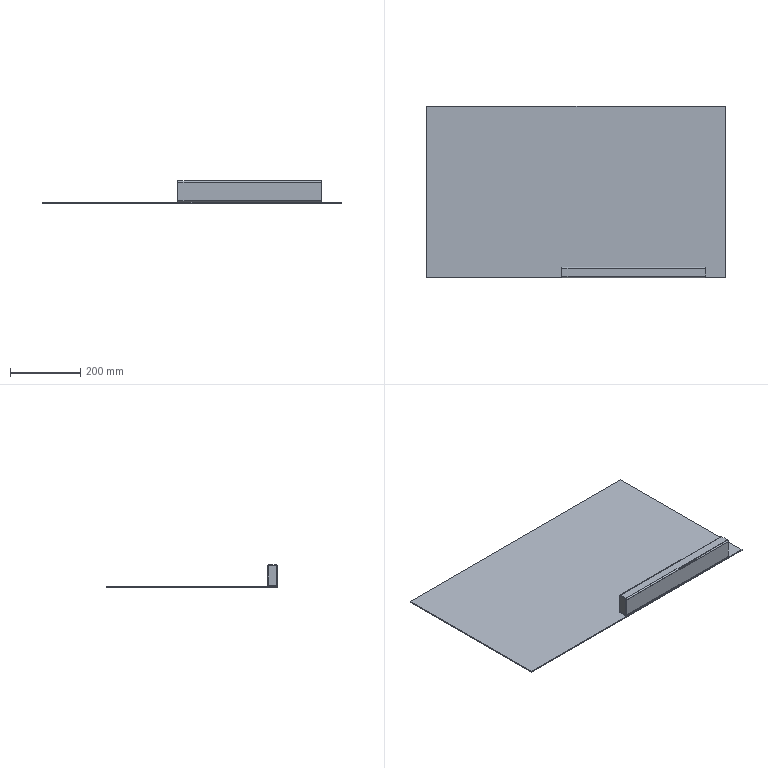Part | SolidWorks | features EndCap 1, Extrusion 1, WeldMemberFeat 1, WeldmentFeature 1 | 3 solids | 34 faces | box 850 x 488 x 63 mm | volume 1385283 mm3 | plane 22 | cylinder 12 | commonest cylinder face diameters 4 x8 8 x4
STEP:
#1=CARTESIAN_POINT('',(425.,-244.,-1.5));
#2=VERTEX_POINT('',#1);
#3=CARTESIAN_POINT('',(425.,244.,-1.5));
#4=VERTEX_POINT('',#3);
#5=CARTESIAN_POINT('',(425.,244.,-1.5));
#6=DIRECTION('',(0.,1.,0.));
#7=VECTOR('',#6,1000.);
#8=LINE('',#5,#7);
#9=EDGE_CURVE('',#2,#4,#8,.T.);
#10=ORIENTED_EDGE('',*,*,#9,.T.);
#11=CARTESIAN_POINT('',(425.,244.,1.5));
#12=VERTEX_POINT('',#11);
#13=CARTESIAN_POINT('',(425.,244.,1.5));
#14=DIRECTION('',(0.,0.,-1.));
#15=VECTOR('',#14,1000.);
#16=LINE('',#13,#15);
#17=EDGE_CURVE('',#12,#4,#16,.T.);
#18=ORIENTED_EDGE('',*,*,#17,.F.);
#19=CARTESIAN_POINT('',(425.,-244.,1.5));
#20=VERTEX_POINT('',#19);
#21=CARTESIAN_POINT('',(425.,244.,1.5));
#22=DIRECTION('',(0.,1.,0.));
#23=VECTOR('',#22,1000.);
#24=LINE('',#21,#23);
#25=EDGE_CURVE('',#20,#12,#24,.T.);
#26=ORIENTED_EDGE('',*,*,#25,.F.);
#27=CARTESIAN_POINT('',(425.,-244.,1.5));
#28=DIRECTION('',(0.,0.,-1.));
#29=VECTOR('',#28,1000.);
#30=LINE('',#27,#29);
#31=EDGE_CURVE('',#20,#2,#30,.T.);
#32=ORIENTED_EDGE('',*,*,#31,.T.);
#33=EDGE_LOOP('',(#10,#18,#26,#32));
#34=FACE_OUTER_BOUND('',#33,.T.);
#35=CARTESIAN_POINT('',(425.,244.,1.5));
#36=DIRECTION('',(-1.,0.,0.));
#37=DIRECTION('',(0.,-1.,0.));
#38=AXIS2_PLACEMENT_3D('',#35,#36,#37);
#39=PLANE('',#38);
#40=ADVANCED_FACE('',(#34),#39,.F.);
#41=CARTESIAN_POINT('',(-425.,244.,-1.5));
#42=VERTEX_POINT('',#41);
#43=CARTESIAN_POINT('',(-425.,244.,-1.5));
#44=DIRECTION('',(-1.,0.,0.));
#45=VECTOR('',#44,1000.);
#46=LINE('',#43,#45);
#47=EDGE_CURVE('',#4,#42,#46,.T.);
#48=ORIENTED_EDGE('',*,*,#47,.T.);
#49=CARTESIAN_POINT('',(-425.,244.,1.5));
#50=VERTEX_POINT('',#49);
#51=CARTESIAN_POINT('',(-425.,244.,1.5));
#52=DIRECTION('',(0.,0.,-1.));
#53=VECTOR('',#52,1000.);
#54=LINE('',#51,#53);
#55=EDGE_CURVE('',#50,#42,#54,.T.);
#56=ORIENTED_EDGE('',*,*,#55,.F.);
#57=CARTESIAN_POINT('',(-425.,244.,1.5));
#58=DIRECTION('',(-1.,0.,0.));
#59=VECTOR('',#58,1000.);
#60=LINE('',#57,#59);
#61=EDGE_CURVE('',#12,#50,#60,.T.);
#62=ORIENTED_EDGE('',*,*,#61,.F.);
#63=ORIENTED_EDGE('',*,*,#17,.T.);
#64=EDGE_LOOP('',(#48,#56,#62,#63));
#65=FACE_OUTER_BOUND('',#64,.T.);
#66=CARTESIAN_POINT('',(-425.,244.,1.5));
#67=DIRECTION('',(0.,-1.,0.));
#68=DIRECTION('',(0.,0.,-1.));
#69=AXIS2_PLACEMENT_3D('',#66,#67,#68);
#70=PLANE('',#69);
#71=ADVANCED_FACE('',(#65),#70,.F.);
#72=CARTESIAN_POINT('',(-425.,-244.,-1.5));
#73=VERTEX_POINT('',#72);
#74=CARTESIAN_POINT('',(-425.,244.,-1.5));
#75=DIRECTION('',(0.,-1.,0.));
#76=VECTOR('',#75,1000.);
#77=LINE('',#74,#76);
#78=EDGE_CURVE('',#42,#73,#77,.T.);
#79=ORIENTED_EDGE('',*,*,#78,.T.);
#80=CARTESIAN_POINT('',(-425.,-244.,1.5));
#81=VERTEX_POINT('',#80);
#82=CARTESIAN_POINT('',(-425.,-244.,1.5));
#83=DIRECTION('',(0.,0.,-1.));
#84=VECTOR('',#83,1000.);
#85=LINE('',#82,#84);
#86=EDGE_CURVE('',#81,#73,#85,.T.);
#87=ORIENTED_EDGE('',*,*,#86,.F.);
#88=CARTESIAN_POINT('',(-425.,244.,1.5));
#89=DIRECTION('',(0.,-1.,0.));
#90=VECTOR('',#89,1000.);
#91=LINE('',#88,#90);
#92=EDGE_CURVE('',#50,#81,#91,.T.);
#93=ORIENTED_EDGE('',*,*,#92,.F.);
#94=ORIENTED_EDGE('',*,*,#55,.T.);
#95=EDGE_LOOP('',(#79,#87,#93,#94));
#96=FACE_OUTER_BOUND('',#95,.T.);
#97=CARTESIAN_POINT('',(-425.,244.,1.5));
#98=DIRECTION('',(1.,0.,0.));
#99=DIRECTION('',(0.,1.,0.));
#100=AXIS2_PLACEMENT_3D('',#97,#98,#99);
#101=PLANE('',#100);
#102=ADVANCED_FACE('',(#96),#101,.F.);
#103=CARTESIAN_POINT('',(-425.,-244.,-1.5));
#104=DIRECTION('',(1.,0.,0.));
#105=VECTOR('',#104,1000.);
#106=LINE('',#103,#105);
#107=EDGE_CURVE('',#73,#2,#106,.T.);
#108=ORIENTED_EDGE('',*,*,#107,.T.);
#109=ORIENTED_EDGE('',*,*,#31,.F.);
#110=CARTESIAN_POINT('',(-425.,-244.,1.5));
#111=DIRECTION('',(1.,0.,0.));
#112=VECTOR('',#111,1000.);
#113=LINE('',#110,#112);
#114=EDGE_CURVE('',#81,#20,#113,.T.);
#115=ORIENTED_EDGE('',*,*,#114,.F.);
#116=ORIENTED_EDGE('',*,*,#86,.T.);
#117=EDGE_LOOP('',(#108,#109,#115,#116));
#118=FACE_OUTER_BOUND('',#117,.T.);
#119=CARTESIAN_POINT('',(-425.,-244.,1.5));
#120=DIRECTION('',(0.,1.,0.));
#121=DIRECTION('',(0.,0.,1.));
#122=AXIS2_PLACEMENT_3D('',#119,#120,#121);
#123=PLANE('',#122);
#124=ADVANCED_FACE('',(#118),#123,.F.);
#125=ORIENTED_EDGE('',*,*,#25,.T.);
#126=ORIENTED_EDGE('',*,*,#61,.T.);
#127=ORIENTED_EDGE('',*,*,#92,.T.);
#128=ORIENTED_EDGE('',*,*,#114,.T.);
#129=EDGE_LOOP('',(#125,#126,#127,#128));
#130=FACE_OUTER_BOUND('',#129,.T.);
#131=CARTESIAN_POINT('',(0.,0.,1.5));
#132=DIRECTION('',(0.,0.,1.));
#133=DIRECTION('',(1.,0.,0.));
#134=AXIS2_PLACEMENT_3D('',#131,#132,#133);
#135=PLANE('',#134);
#136=ADVANCED_FACE('',(#130),#135,.T.);
#137=ORIENTED_EDGE('',*,*,#9,.F.);
#138=ORIENTED_EDGE('',*,*,#107,.F.);
#139=ORIENTED_EDGE('',*,*,#78,.F.);
#140=ORIENTED_EDGE('',*,*,#47,.F.);
#141=EDGE_LOOP('',(#137,#138,#139,#140));
#142=FACE_OUTER_BOUND('',#141,.T.);
#143=CARTESIAN_POINT('',(0.,0.,-1.5));
#144=DIRECTION('',(0.,0.,1.));
#145=DIRECTION('',(1.,0.,0.));
#146=AXIS2_PLACEMENT_3D('',#143,#144,#145);
#147=PLANE('',#146);
#148=ADVANCED_FACE('',(#142),#147,.F.);
#149=CLOSED_SHELL('',(#40,#71,#102,#124,#136,#148));
#150=MANIFOLD_SOLID_BREP('',#149);
#151=CARTESIAN_POINT('',(370.,-244.,57.5));
#152=VERTEX_POINT('',#151);
#153=CARTESIAN_POINT('',(370.,-240.,61.5));
#154=VERTEX_POINT('',#153);
#155=CARTESIAN_POINT('',(370.,-240.,57.5));
#156=DIRECTION('',(-1.,0.,0.));
#157=DIRECTION('',(0.,-1.,0.));
#158=AXIS2_PLACEMENT_3D('',#155,#156,#157);
#159=CIRCLE('',#158,4.);
#160=EDGE_CURVE('',#152,#154,#159,.T.);
#161=ORIENTED_EDGE('',*,*,#160,.T.);
#162=CARTESIAN_POINT('',(-40.,-240.,61.5));
#163=VERTEX_POINT('',#162);
#164=CARTESIAN_POINT('',(-40.,-240.,61.5));
#165=DIRECTION('',(1.,0.,0.));
#166=VECTOR('',#165,1000.);
#167=LINE('',#164,#166);
#168=EDGE_CURVE('',#163,#154,#167,.T.);
#169=ORIENTED_EDGE('',*,*,#168,.F.);
#170=CARTESIAN_POINT('',(-40.,-244.,57.5));
#171=VERTEX_POINT('',#170);
#172=CARTESIAN_POINT('',(-40.,-240.,57.5));
#173=DIRECTION('',(-1.,0.,0.));
#174=DIRECTION('',(0.,-1.,0.));
#175=AXIS2_PLACEMENT_3D('',#172,#173,#174);
#176=CIRCLE('',#175,4.);
#177=EDGE_CURVE('',#171,#163,#176,.T.);
#178=ORIENTED_EDGE('',*,*,#177,.F.);
#179=CARTESIAN_POINT('',(-40.,-244.,57.5));
#180=DIRECTION('',(1.,0.,0.));
#181=VECTOR('',#180,1000.);
#182=LINE('',#179,#181);
#183=EDGE_CURVE('',#171,#152,#182,.T.);
#184=ORIENTED_EDGE('',*,*,#183,.T.);
#185=EDGE_LOOP('',(#161,#169,#178,#184));
#186=FACE_OUTER_BOUND('',#185,.T.);
#187=CARTESIAN_POINT('',(-40.,-240.,57.5));
#188=DIRECTION('',(1.,0.,0.));
#189=DIRECTION('',(0.,1.,0.));
#190=AXIS2_PLACEMENT_3D('',#187,#188,#189);
#191=CYLINDRICAL_SURFACE('',#190,4.);
#192=ADVANCED_FACE('',(#186),#191,.T.);
#193=CARTESIAN_POINT('',(370.,-218.,61.5));
#194=VERTEX_POINT('',#193);
#195=CARTESIAN_POINT('',(370.,-240.,61.5));
#196=DIRECTION('',(0.,1.,0.));
#197=VECTOR('',#196,1000.);
#198=LINE('',#195,#197);
#199=EDGE_CURVE('',#154,#194,#198,.T.);
#200=ORIENTED_EDGE('',*,*,#199,.T.);
#201=CARTESIAN_POINT('',(-40.,-218.,61.5));
#202=VERTEX_POINT('',#201);
#203=CARTESIAN_POINT('',(-40.,-218.,61.5));
#204=DIRECTION('',(1.,0.,0.));
#205=VECTOR('',#204,1000.);
#206=LINE('',#203,#205);
#207=EDGE_CURVE('',#202,#194,#206,.T.);
#208=ORIENTED_EDGE('',*,*,#207,.F.);
#209=CARTESIAN_POINT('',(-40.,-240.,61.5));
#210=DIRECTION('',(0.,1.,0.));
#211=VECTOR('',#210,1000.);
#212=LINE('',#209,#211);
#213=EDGE_CURVE('',#163,#202,#212,.T.);
#214=ORIENTED_EDGE('',*,*,#213,.F.);
#215=ORIENTED_EDGE('',*,*,#168,.T.);
#216=EDGE_LOOP('',(#200,#208,#214,#215));
#217=FACE_OUTER_BOUND('',#216,.T.);
#218=CARTESIAN_POINT('',(-40.,-240.,61.5));
#219=DIRECTION('',(0.,0.,-1.));
#220=DIRECTION('',(-1.,0.,0.));
#221=AXIS2_PLACEMENT_3D('',#218,#219,#220);
#222=PLANE('',#221);
#223=ADVANCED_FACE('',(#217),#222,.F.);
#224=CARTESIAN_POINT('',(370.,-214.,57.5));
#225=VERTEX_POINT('',#224);
#226=CARTESIAN_POINT('',(370.,-218.,57.5));
#227=DIRECTION('',(-1.,0.,0.));
#228=DIRECTION('',(0.,-1.,0.));
#229=AXIS2_PLACEMENT_3D('',#226,#227,#228);
#230=CIRCLE('',#229,4.);
#231=EDGE_CURVE('',#194,#225,#230,.T.);
#232=ORIENTED_EDGE('',*,*,#231,.T.);
#233=CARTESIAN_POINT('',(-40.,-214.,57.5));
#234=VERTEX_POINT('',#233);
#235=CARTESIAN_POINT('',(-40.,-214.,57.5));
#236=DIRECTION('',(1.,0.,0.));
#237=VECTOR('',#236,1000.);
#238=LINE('',#235,#237);
#239=EDGE_CURVE('',#234,#225,#238,.T.);
#240=ORIENTED_EDGE('',*,*,#239,.F.);
#241=CARTESIAN_POINT('',(-40.,-218.,57.5));
#242=DIRECTION('',(-1.,0.,0.));
#243=DIRECTION('',(0.,-1.,0.));
#244=AXIS2_PLACEMENT_3D('',#241,#242,#243);
#245=CIRCLE('',#244,4.);
#246=EDGE_CURVE('',#202,#234,#245,.T.);
#247=ORIENTED_EDGE('',*,*,#246,.F.);
#248=ORIENTED_EDGE('',*,*,#207,.T.);
#249=EDGE_LOOP('',(#232,#240,#247,#248));
#250=FACE_OUTER_BOUND('',#249,.T.);
#251=CARTESIAN_POINT('',(-40.,-218.,57.5));
#252=DIRECTION('',(1.,0.,0.));
#253=DIRECTION('',(0.,1.,0.));
#254=AXIS2_PLACEMENT_3D('',#251,#252,#253);
#255=CYLINDRICAL_SURFACE('',#254,4.);
#256=ADVANCED_FACE('',(#250),#255,.T.);
#257=CARTESIAN_POINT('',(370.,-214.,5.5));
#258=VERTEX_POINT('',#257);
#259=CARTESIAN_POINT('',(370.,-214.,5.5));
#260=DIRECTION('',(0.,0.,-1.));
#261=VECTOR('',#260,1000.);
#262=LINE('',#259,#261);
#263=EDGE_CURVE('',#225,#258,#262,.T.);
#264=ORIENTED_EDGE('',*,*,#263,.T.);
#265=CARTESIAN_POINT('',(-40.,-214.,5.5));
#266=VERTEX_POINT('',#265);
#267=CARTESIAN_POINT('',(-40.,-214.,5.5));
#268=DIRECTION('',(1.,0.,0.));
#269=VECTOR('',#268,1000.);
#270=LINE('',#267,#269);
#271=EDGE_CURVE('',#266,#258,#270,.T.);
#272=ORIENTED_EDGE('',*,*,#271,.F.);
#273=CARTESIAN_POINT('',(-40.,-214.,5.5));
#274=DIRECTION('',(0.,0.,-1.));
#275=VECTOR('',#274,1000.);
#276=LINE('',#273,#275);
#277=EDGE_CURVE('',#234,#266,#276,.T.);
#278=ORIENTED_EDGE('',*,*,#277,.F.);
#279=ORIENTED_EDGE('',*,*,#239,.T.);
#280=EDGE_LOOP('',(#264,#272,#278,#279));
#281=FACE_OUTER_BOUND('',#280,.T.);
#282=CARTESIAN_POINT('',(-40.,-214.,5.5));
#283=DIRECTION('',(0.,-1.,0.));
#284=DIRECTION('',(1.,0.,0.));
#285=AXIS2_PLACEMENT_3D('',#282,#283,#284);
#286=PLANE('',#285);
#287=ADVANCED_FACE('',(#281),#286,.F.);
#288=CARTESIAN_POINT('',(370.,-218.,1.5));
#289=VERTEX_POINT('',#288);
#290=CARTESIAN_POINT('',(370.,-218.,5.5));
#291=DIRECTION('',(-1.,0.,0.));
#292=DIRECTION('',(0.,-1.,0.));
#293=AXIS2_PLACEMENT_3D('',#290,#291,#292);
#294=CIRCLE('',#293,4.);
#295=EDGE_CURVE('',#258,#289,#294,.T.);
#296=ORIENTED_EDGE('',*,*,#295,.T.);
#297=CARTESIAN_POINT('',(-40.,-218.,1.5));
#298=VERTEX_POINT('',#297);
#299=CARTESIAN_POINT('',(-40.,-218.,1.5));
#300=DIRECTION('',(1.,0.,0.));
#301=VECTOR('',#300,1000.);
#302=LINE('',#299,#301);
#303=EDGE_CURVE('',#298,#289,#302,.T.);
#304=ORIENTED_EDGE('',*,*,#303,.F.);
#305=CARTESIAN_POINT('',(-40.,-218.,5.5));
#306=DIRECTION('',(-1.,0.,0.));
#307=DIRECTION('',(0.,-1.,0.));
#308=AXIS2_PLACEMENT_3D('',#305,#306,#307);
#309=CIRCLE('',#308,4.);
#310=EDGE_CURVE('',#266,#298,#309,.T.);
#311=ORIENTED_EDGE('',*,*,#310,.F.);
#312=ORIENTED_EDGE('',*,*,#271,.T.);
#313=EDGE_LOOP('',(#296,#304,#311,#312));
#314=FACE_OUTER_BOUND('',#313,.T.);
#315=CARTESIAN_POINT('',(-40.,-218.,5.5));
#316=DIRECTION('',(1.,0.,0.));
#317=DIRECTION('',(0.,1.,0.));
#318=AXIS2_PLACEMENT_3D('',#315,#316,#317);
#319=CYLINDRICAL_SURFACE('',#318,4.);
#320=ADVANCED_FACE('',(#314),#319,.T.);
#321=CARTESIAN_POINT('',(370.,-240.,1.5));
#322=VERTEX_POINT('',#321);
#323=CARTESIAN_POINT('',(370.,-218.,1.5));
#324=DIRECTION('',(0.,-1.,0.));
#325=VECTOR('',#324,1000.);
#326=LINE('',#323,#325);
#327=EDGE_CURVE('',#289,#322,#326,.T.);
#328=ORIENTED_EDGE('',*,*,#327,.T.);
#329=CARTESIAN_POINT('',(-40.,-240.,1.5));
#330=VERTEX_POINT('',#329);
#331=CARTESIAN_POINT('',(-40.,-240.,1.5));
#332=DIRECTION('',(1.,0.,0.));
#333=VECTOR('',#332,1000.);
#334=LINE('',#331,#333);
#335=EDGE_CURVE('',#330,#322,#334,.T.);
#336=ORIENTED_EDGE('',*,*,#335,.F.);
#337=CARTESIAN_POINT('',(-40.,-218.,1.5));
#338=DIRECTION('',(0.,-1.,0.));
#339=VECTOR('',#338,1000.);
#340=LINE('',#337,#339);
#341=EDGE_CURVE('',#298,#330,#340,.T.);
#342=ORIENTED_EDGE('',*,*,#341,.F.);
#343=ORIENTED_EDGE('',*,*,#303,.T.);
#344=EDGE_LOOP('',(#328,#336,#342,#343));
#345=FACE_OUTER_BOUND('',#344,.T.);
#346=CARTESIAN_POINT('',(-40.,-218.,1.5));
#347=DIRECTION('',(0.,0.,1.));
#348=DIRECTION('',(1.,0.,0.));
#349=AXIS2_PLACEMENT_3D('',#346,#347,#348);
#350=PLANE('',#349);
#351=ADVANCED_FACE('',(#345),#350,.F.);
#352=CARTESIAN_POINT('',(370.,-244.,5.5));
#353=VERTEX_POINT('',#352);
#354=CARTESIAN_POINT('',(370.,-240.,5.5));
#355=DIRECTION('',(-1.,0.,0.));
#356=DIRECTION('',(0.,-1.,0.));
#357=AXIS2_PLACEMENT_3D('',#354,#355,#356);
#358=CIRCLE('',#357,4.);
#359=EDGE_CURVE('',#322,#353,#358,.T.);
#360=ORIENTED_EDGE('',*,*,#359,.T.);
#361=CARTESIAN_POINT('',(-40.,-244.,5.5));
#362=VERTEX_POINT('',#361);
#363=CARTESIAN_POINT('',(-40.,-244.,5.5));
#364=DIRECTION('',(1.,0.,0.));
#365=VECTOR('',#364,1000.);
#366=LINE('',#363,#365);
#367=EDGE_CURVE('',#362,#353,#366,.T.);
#368=ORIENTED_EDGE('',*,*,#367,.F.);
#369=CARTESIAN_POINT('',(-40.,-240.,5.5));
#370=DIRECTION('',(-1.,0.,0.));
#371=DIRECTION('',(0.,-1.,0.));
#372=AXIS2_PLACEMENT_3D('',#369,#370,#371);
#373=CIRCLE('',#372,4.);
#374=EDGE_CURVE('',#330,#362,#373,.T.);
#375=ORIENTED_EDGE('',*,*,#374,.F.);
#376=ORIENTED_EDGE('',*,*,#335,.T.);
#377=EDGE_LOOP('',(#360,#368,#375,#376));
#378=FACE_OUTER_BOUND('',#377,.T.);
#379=CARTESIAN_POINT('',(-40.,-240.,5.5));
#380=DIRECTION('',(1.,0.,0.));
#381=DIRECTION('',(0.,1.,0.));
#382=AXIS2_PLACEMENT_3D('',#379,#380,#381);
#383=CYLINDRICAL_SURFACE('',#382,4.);
#384=ADVANCED_FACE('',(#378),#383,.T.);
#385=CARTESIAN_POINT('',(370.,-218.,59.5));
#386=VERTEX_POINT('',#385);
#387=CARTESIAN_POINT('',(370.,-216.,57.5));
#388=VERTEX_POINT('',#387);
#389=CARTESIAN_POINT('',(370.,-218.,57.5));
#390=DIRECTION('',(-1.,0.,0.));
#391=DIRECTION('',(0.,-1.,0.));
#392=AXIS2_PLACEMENT_3D('',#389,#390,#391);
#393=CIRCLE('',#392,2.);
#394=EDGE_CURVE('',#386,#388,#393,.T.);
#395=ORIENTED_EDGE('',*,*,#394,.F.);
#396=CARTESIAN_POINT('',(-40.,-218.,59.5));
#397=VERTEX_POINT('',#396);
#398=CARTESIAN_POINT('',(-40.,-218.,59.5));
#399=DIRECTION('',(1.,0.,0.));
#400=VECTOR('',#399,1000.);
#401=LINE('',#398,#400);
#402=EDGE_CURVE('',#397,#386,#401,.T.);
#403=ORIENTED_EDGE('',*,*,#402,.F.);
#404=CARTESIAN_POINT('',(-40.,-216.,57.5));
#405=VERTEX_POINT('',#404);
#406=CARTESIAN_POINT('',(-40.,-218.,57.5));
#407=DIRECTION('',(-1.,0.,0.));
#408=DIRECTION('',(0.,-1.,0.));
#409=AXIS2_PLACEMENT_3D('',#406,#407,#408);
#410=CIRCLE('',#409,2.);
#411=EDGE_CURVE('',#397,#405,#410,.T.);
#412=ORIENTED_EDGE('',*,*,#411,.T.);
#413=CARTESIAN_POINT('',(-40.,-216.,57.5));
#414=DIRECTION('',(1.,0.,0.));
#415=VECTOR('',#414,1000.);
#416=LINE('',#413,#415);
#417=EDGE_CURVE('',#405,#388,#416,.T.);
#418=ORIENTED_EDGE('',*,*,#417,.T.);
#419=EDGE_LOOP('',(#395,#403,#412,#418));
#420=FACE_OUTER_BOUND('',#419,.T.);
#421=CARTESIAN_POINT('',(-40.,-218.,57.5));
#422=DIRECTION('',(1.,0.,0.));
#423=DIRECTION('',(0.,1.,0.));
#424=AXIS2_PLACEMENT_3D('',#421,#422,#423);
#425=CYLINDRICAL_SURFACE('',#424,2.);
#426=ADVANCED_FACE('',(#420),#425,.F.);
#427=CARTESIAN_POINT('',(370.,-240.,59.5));
#428=VERTEX_POINT('',#427);
#429=CARTESIAN_POINT('',(370.,-240.,59.5));
#430=DIRECTION('',(0.,1.,0.));
#431=VECTOR('',#430,1000.);
#432=LINE('',#429,#431);
#433=EDGE_CURVE('',#428,#386,#432,.T.);
#434=ORIENTED_EDGE('',*,*,#433,.F.);
#435=CARTESIAN_POINT('',(-40.,-240.,59.5));
#436=VERTEX_POINT('',#435);
#437=CARTESIAN_POINT('',(-40.,-240.,59.5));
#438=DIRECTION('',(1.,0.,0.));
#439=VECTOR('',#438,1000.);
#440=LINE('',#437,#439);
#441=EDGE_CURVE('',#436,#428,#440,.T.);
#442=ORIENTED_EDGE('',*,*,#441,.F.);
#443=CARTESIAN_POINT('',(-40.,-240.,59.5));
#444=DIRECTION('',(0.,1.,0.));
#445=VECTOR('',#444,1000.);
#446=LINE('',#443,#445);
#447=EDGE_CURVE('',#436,#397,#446,.T.);
#448=ORIENTED_EDGE('',*,*,#447,.T.);
#449=ORIENTED_EDGE('',*,*,#402,.T.);
#450=EDGE_LOOP('',(#434,#442,#448,#449));
#451=FACE_OUTER_BOUND('',#450,.T.);
#452=CARTESIAN_POINT('',(-40.,-240.,59.5));
#453=DIRECTION('',(0.,0.,-1.));
#454=DIRECTION('',(-1.,0.,0.));
#455=AXIS2_PLACEMENT_3D('',#452,#453,#454);
#456=PLANE('',#455);
#457=ADVANCED_FACE('',(#451),#456,.T.);
#458=CARTESIAN_POINT('',(370.,-242.,57.5));
#459=VERTEX_POINT('',#458);
#460=CARTESIAN_POINT('',(370.,-240.,57.5));
#461=DIRECTION('',(-1.,0.,0.));
#462=DIRECTION('',(0.,-1.,0.));
#463=AXIS2_PLACEMENT_3D('',#460,#461,#462);
#464=CIRCLE('',#463,2.);
#465=EDGE_CURVE('',#459,#428,#464,.T.);
#466=ORIENTED_EDGE('',*,*,#465,.F.);
#467=CARTESIAN_POINT('',(-40.,-242.,57.5));
#468=VERTEX_POINT('',#467);
#469=CARTESIAN_POINT('',(-40.,-242.,57.5));
#470=DIRECTION('',(1.,0.,0.));
#471=VECTOR('',#470,1000.);
#472=LINE('',#469,#471);
#473=EDGE_CURVE('',#468,#459,#472,.T.);
#474=ORIENTED_EDGE('',*,*,#473,.F.);
#475=CARTESIAN_POINT('',(-40.,-240.,57.5));
#476=DIRECTION('',(-1.,0.,0.));
#477=DIRECTION('',(0.,-1.,0.));
#478=AXIS2_PLACEMENT_3D('',#475,#476,#477);
#479=CIRCLE('',#478,2.);
#480=EDGE_CURVE('',#468,#436,#479,.T.);
#481=ORIENTED_EDGE('',*,*,#480,.T.);
#482=ORIENTED_EDGE('',*,*,#441,.T.);
#483=EDGE_LOOP('',(#466,#474,#481,#482));
#484=FACE_OUTER_BOUND('',#483,.T.);
#485=CARTESIAN_POINT('',(-40.,-240.,57.5));
#486=DIRECTION('',(1.,0.,0.));
#487=DIRECTION('',(0.,1.,0.));
#488=AXIS2_PLACEMENT_3D('',#485,#486,#487);
#489=CYLINDRICAL_SURFACE('',#488,2.);
#490=ADVANCED_FACE('',(#484),#489,.F.);
#491=CARTESIAN_POINT('',(370.,-242.,5.5));
#492=VERTEX_POINT('',#491);
#493=CARTESIAN_POINT('',(370.,-242.,57.5));
#494=DIRECTION('',(0.,0.,1.));
#495=VECTOR('',#494,1000.);
#496=LINE('',#493,#495);
#497=EDGE_CURVE('',#492,#459,#496,.T.);
#498=ORIENTED_EDGE('',*,*,#497,.F.);
#499=CARTESIAN_POINT('',(-40.,-242.,5.5));
#500=VERTEX_POINT('',#499);
#501=CARTESIAN_POINT('',(-40.,-242.,5.5));
#502=DIRECTION('',(1.,0.,0.));
#503=VECTOR('',#502,1000.);
#504=LINE('',#501,#503);
#505=EDGE_CURVE('',#500,#492,#504,.T.);
#506=ORIENTED_EDGE('',*,*,#505,.F.);
#507=CARTESIAN_POINT('',(-40.,-242.,57.5));
#508=DIRECTION('',(0.,0.,1.));
#509=VECTOR('',#508,1000.);
#510=LINE('',#507,#509);
#511=EDGE_CURVE('',#500,#468,#510,.T.);
#512=ORIENTED_EDGE('',*,*,#511,.T.);
#513=ORIENTED_EDGE('',*,*,#473,.T.);
#514=EDGE_LOOP('',(#498,#506,#512,#513));
#515=FACE_OUTER_BOUND('',#514,.T.);
#516=CARTESIAN_POINT('',(-40.,-242.,57.5));
#517=DIRECTION('',(0.,1.,0.));
#518=DIRECTION('',(-1.,0.,0.));
#519=AXIS2_PLACEMENT_3D('',#516,#517,#518);
#520=PLANE('',#519);
#521=ADVANCED_FACE('',(#515),#520,.T.);
#522=CARTESIAN_POINT('',(370.,-240.,3.5));
#523=VERTEX_POINT('',#522);
#524=CARTESIAN_POINT('',(370.,-240.,5.5));
#525=DIRECTION('',(-1.,0.,0.));
#526=DIRECTION('',(0.,-1.,0.));
#527=AXIS2_PLACEMENT_3D('',#524,#525,#526);
#528=CIRCLE('',#527,2.);
#529=EDGE_CURVE('',#523,#492,#528,.T.);
#530=ORIENTED_EDGE('',*,*,#529,.F.);
#531=CARTESIAN_POINT('',(-40.,-240.,3.5));
#532=VERTEX_POINT('',#531);
#533=CARTESIAN_POINT('',(-40.,-240.,3.5));
#534=DIRECTION('',(1.,0.,0.));
#535=VECTOR('',#534,1000.);
#536=LINE('',#533,#535);
#537=EDGE_CURVE('',#532,#523,#536,.T.);
#538=ORIENTED_EDGE('',*,*,#537,.F.);
#539=CARTESIAN_POINT('',(-40.,-240.,5.5));
#540=DIRECTION('',(-1.,0.,0.));
#541=DIRECTION('',(0.,-1.,0.));
#542=AXIS2_PLACEMENT_3D('',#539,#540,#541);
#543=CIRCLE('',#542,2.);
#544=EDGE_CURVE('',#532,#500,#543,.T.);
#545=ORIENTED_EDGE('',*,*,#544,.T.);
#546=ORIENTED_EDGE('',*,*,#505,.T.);
#547=EDGE_LOOP('',(#530,#538,#545,#546));
#548=FACE_OUTER_BOUND('',#547,.T.);
#549=CARTESIAN_POINT('',(-40.,-240.,5.5));
#550=DIRECTION('',(1.,0.,0.));
#551=DIRECTION('',(0.,1.,0.));
#552=AXIS2_PLACEMENT_3D('',#549,#550,#551);
#553=CYLINDRICAL_SURFACE('',#552,2.);
#554=ADVANCED_FACE('',(#548),#553,.F.);
#555=CARTESIAN_POINT('',(370.,-218.,3.5));
#556=VERTEX_POINT('',#555);
#557=CARTESIAN_POINT('',(370.,-218.,3.5));
#558=DIRECTION('',(0.,-1.,0.));
#559=VECTOR('',#558,1000.);
#560=LINE('',#557,#559);
#561=EDGE_CURVE('',#556,#523,#560,.T.);
#562=ORIENTED_EDGE('',*,*,#561,.F.);
#563=CARTESIAN_POINT('',(-40.,-218.,3.5));
#564=VERTEX_POINT('',#563);
#565=CARTESIAN_POINT('',(-40.,-218.,3.5));
#566=DIRECTION('',(1.,0.,0.));
#567=VECTOR('',#566,1000.);
#568=LINE('',#565,#567);
#569=EDGE_CURVE('',#564,#556,#568,.T.);
#570=ORIENTED_EDGE('',*,*,#569,.F.);
#571=CARTESIAN_POINT('',(-40.,-218.,3.5));
#572=DIRECTION('',(0.,-1.,0.));
#573=VECTOR('',#572,1000.);
#574=LINE('',#571,#573);
#575=EDGE_CURVE('',#564,#532,#574,.T.);
#576=ORIENTED_EDGE('',*,*,#575,.T.);
#577=ORIENTED_EDGE('',*,*,#537,.T.);
#578=EDGE_LOOP('',(#562,#570,#576,#577));
#579=FACE_OUTER_BOUND('',#578,.T.);
#580=CARTESIAN_POINT('',(-40.,-218.,3.5));
#581=DIRECTION('',(0.,0.,1.));
#582=DIRECTION('',(1.,0.,0.));
#583=AXIS2_PLACEMENT_3D('',#580,#581,#582);
#584=PLANE('',#583);
#585=ADVANCED_FACE('',(#579),#584,.T.);
#586=CARTESIAN_POINT('',(370.,-216.,5.5));
#587=VERTEX_POINT('',#586);
#588=CARTESIAN_POINT('',(370.,-218.,5.5));
#589=DIRECTION('',(-1.,0.,0.));
#590=DIRECTION('',(0.,-1.,0.));
#591=AXIS2_PLACEMENT_3D('',#588,#589,#590);
#592=CIRCLE('',#591,2.);
#593=EDGE_CURVE('',#587,#556,#592,.T.);
#594=ORIENTED_EDGE('',*,*,#593,.F.);
#595=CARTESIAN_POINT('',(-40.,-216.,5.5));
#596=VERTEX_POINT('',#595);
#597=CARTESIAN_POINT('',(-40.,-216.,5.5));
#598=DIRECTION('',(1.,0.,0.));
#599=VECTOR('',#598,1000.);
#600=LINE('',#597,#599);
#601=EDGE_CURVE('',#596,#587,#600,.T.);
#602=ORIENTED_EDGE('',*,*,#601,.F.);
#603=CARTESIAN_POINT('',(-40.,-218.,5.5));
#604=DIRECTION('',(-1.,0.,0.));
#605=DIRECTION('',(0.,-1.,0.));
#606=AXIS2_PLACEMENT_3D('',#603,#604,#605);
#607=CIRCLE('',#606,2.);
#608=EDGE_CURVE('',#596,#564,#607,.T.);
#609=ORIENTED_EDGE('',*,*,#608,.T.);
#610=ORIENTED_EDGE('',*,*,#569,.T.);
#611=EDGE_LOOP('',(#594,#602,#609,#610));
#612=FACE_OUTER_BOUND('',#611,.T.);
#613=CARTESIAN_POINT('',(-40.,-218.,5.5));
#614=DIRECTION('',(1.,0.,0.));
#615=DIRECTION('',(0.,1.,0.));
#616=AXIS2_PLACEMENT_3D('',#613,#614,#615);
#617=CYLINDRICAL_SURFACE('',#616,2.);
#618=ADVANCED_FACE('',(#612),#617,.F.);
#619=CARTESIAN_POINT('',(370.,-216.,5.5));
#620=DIRECTION('',(0.,0.,-1.));
#621=VECTOR('',#620,1000.);
#622=LINE('',#619,#621);
#623=EDGE_CURVE('',#388,#587,#622,.T.);
#624=ORIENTED_EDGE('',*,*,#623,.F.);
#625=ORIENTED_EDGE('',*,*,#417,.F.);
#626=CARTESIAN_POINT('',(-40.,-216.,5.5));
#627=DIRECTION('',(0.,0.,-1.));
#628=VECTOR('',#627,1000.);
#629=LINE('',#626,#628);
#630=EDGE_CURVE('',#405,#596,#629,.T.);
#631=ORIENTED_EDGE('',*,*,#630,.T.);
#632=ORIENTED_EDGE('',*,*,#601,.T.);
#633=EDGE_LOOP('',(#624,#625,#631,#632));
#634=FACE_OUTER_BOUND('',#633,.T.);
#635=CARTESIAN_POINT('',(-40.,-216.,5.5));
#636=DIRECTION('',(0.,-1.,0.));
#637=DIRECTION('',(1.,0.,0.));
#638=AXIS2_PLACEMENT_3D('',#635,#636,#637);
#639=PLANE('',#638);
#640=ADVANCED_FACE('',(#634),#639,.T.);
#641=CARTESIAN_POINT('',(370.,-244.,57.5));
#642=DIRECTION('',(0.,0.,1.));
#643=VECTOR('',#642,1000.);
#644=LINE('',#641,#643);
#645=EDGE_CURVE('',#353,#152,#644,.T.);
#646=ORIENTED_EDGE('',*,*,#645,.T.);
#647=ORIENTED_EDGE('',*,*,#183,.F.);
#648=CARTESIAN_POINT('',(-40.,-244.,57.5));
#649=DIRECTION('',(0.,0.,1.));
#650=VECTOR('',#649,1000.);
#651=LINE('',#648,#650);
#652=EDGE_CURVE('',#362,#171,#651,.T.);
#653=ORIENTED_EDGE('',*,*,#652,.F.);
#654=ORIENTED_EDGE('',*,*,#367,.T.);
#655=EDGE_LOOP('',(#646,#647,#653,#654));
#656=FACE_OUTER_BOUND('',#655,.T.);
#657=CARTESIAN_POINT('',(-40.,-244.,57.5));
#658=DIRECTION('',(0.,1.,0.));
#659=DIRECTION('',(-1.,0.,0.));
#660=AXIS2_PLACEMENT_3D('',#657,#658,#659);
#661=PLANE('',#660);
#662=ADVANCED_FACE('',(#656),#661,.F.);
#663=ORIENTED_EDGE('',*,*,#411,.F.);
#664=ORIENTED_EDGE('',*,*,#447,.F.);
#665=ORIENTED_EDGE('',*,*,#480,.F.);
#666=ORIENTED_EDGE('',*,*,#511,.F.);
#667=ORIENTED_EDGE('',*,*,#544,.F.);
#668=ORIENTED_EDGE('',*,*,#575,.F.);
#669=ORIENTED_EDGE('',*,*,#608,.F.);
#670=ORIENTED_EDGE('',*,*,#630,.F.);
#671=EDGE_LOOP('',(#663,#664,#665,#666,#667,#668,#669,#670));
#672=FACE_BOUND('',#671,.T.);
#673=ORIENTED_EDGE('',*,*,#177,.T.);
#674=ORIENTED_EDGE('',*,*,#213,.T.);
#675=ORIENTED_EDGE('',*,*,#246,.T.);
#676=ORIENTED_EDGE('',*,*,#277,.T.);
#677=ORIENTED_EDGE('',*,*,#310,.T.);
#678=ORIENTED_EDGE('',*,*,#341,.T.);
#679=ORIENTED_EDGE('',*,*,#374,.T.);
#680=ORIENTED_EDGE('',*,*,#652,.T.);
#681=EDGE_LOOP('',(#673,#674,#675,#676,#677,#678,#679,#680));
#682=FACE_OUTER_BOUND('',#681,.T.);
#683=CARTESIAN_POINT('',(-40.,-240.,57.5));
#684=DIRECTION('',(-1.,0.,0.));
#685=DIRECTION('',(0.,-1.,0.));
#686=AXIS2_PLACEMENT_3D('',#683,#684,#685);
#687=PLANE('',#686);
#688=ADVANCED_FACE('',(#672,#682),#687,.T.);
#689=ORIENTED_EDGE('',*,*,#394,.T.);
#690=ORIENTED_EDGE('',*,*,#623,.T.);
#691=ORIENTED_EDGE('',*,*,#593,.T.);
#692=ORIENTED_EDGE('',*,*,#561,.T.);
#693=ORIENTED_EDGE('',*,*,#529,.T.);
#694=ORIENTED_EDGE('',*,*,#497,.T.);
#695=ORIENTED_EDGE('',*,*,#465,.T.);
#696=ORIENTED_EDGE('',*,*,#433,.T.);
#697=EDGE_LOOP('',(#689,#690,#691,#692,#693,#694,#695,#696));
#698=FACE_BOUND('',#697,.T.);
#699=ORIENTED_EDGE('',*,*,#160,.F.);
#700=ORIENTED_EDGE('',*,*,#645,.F.);
#701=ORIENTED_EDGE('',*,*,#359,.F.);
#702=ORIENTED_EDGE('',*,*,#327,.F.);
#703=ORIENTED_EDGE('',*,*,#295,.F.);
#704=ORIENTED_EDGE('',*,*,#263,.F.);
#705=ORIENTED_EDGE('',*,*,#231,.F.);
#706=ORIENTED_EDGE('',*,*,#199,.F.);
#707=EDGE_LOOP('',(#699,#700,#701,#702,#703,#704,#705,#706));
#708=FACE_OUTER_BOUND('',#707,.T.);
#709=CARTESIAN_POINT('',(370.,-240.,57.5));
#710=DIRECTION('',(-1.,0.,0.));
#711=DIRECTION('',(0.,-1.,0.));
#712=AXIS2_PLACEMENT_3D('',#709,#710,#711);
#713=PLANE('',#712);
#714=ADVANCED_FACE('',(#698,#708),#713,.F.);
#715=CLOSED_SHELL('',(#192,#223,#256,#287,#320,#351,#384,#426,#457,#490,#521,#554,#585,#618,#640,#662,#688,#714));
#716=MANIFOLD_SOLID_BREP('',#715);
#717=CARTESIAN_POINT('',(-40.,-241.4,56.9));
#718=VERTEX_POINT('',#717);
#719=CARTESIAN_POINT('',(-40.,-241.4,6.1));
#720=VERTEX_POINT('',#719);
#721=CARTESIAN_POINT('',(-40.,-241.4,58.9));
#722=DIRECTION('',(0.,0.,-1.));
#723=VECTOR('',#722,1000.);
#724=LINE('',#721,#723);
#725=EDGE_CURVE('',#718,#720,#724,.T.);
#726=ORIENTED_EDGE('',*,*,#725,.T.);
#727=CARTESIAN_POINT('',(-37.,-241.4,6.1));
#728=VERTEX_POINT('',#727);
#729=CARTESIAN_POINT('',(-37.,-241.4,6.1));
#730=DIRECTION('',(-1.,0.,0.));
#731=VECTOR('',#730,1000.);
#732=LINE('',#729,#731);
#733=EDGE_CURVE('',#728,#720,#732,.T.);
#734=ORIENTED_EDGE('',*,*,#733,.F.);
#735=CARTESIAN_POINT('',(-37.,-241.4,56.9));
#736=VERTEX_POINT('',#735);
#737=CARTESIAN_POINT('',(-37.,-241.4,58.9));
#738=DIRECTION('',(0.,0.,-1.));
#739=VECTOR('',#738,1000.);
#740=LINE('',#737,#739);
#741=EDGE_CURVE('',#736,#728,#740,.T.);
#742=ORIENTED_EDGE('',*,*,#741,.F.);
#743=CARTESIAN_POINT('',(-37.,-241.4,56.9));
#744=DIRECTION('',(-1.,0.,0.));
#745=VECTOR('',#744,1000.);
#746=LINE('',#743,#745);
#747=EDGE_CURVE('',#736,#718,#746,.T.);
#748=ORIENTED_EDGE('',*,*,#747,.T.);
#749=EDGE_LOOP('',(#726,#734,#742,#748));
#750=FACE_OUTER_BOUND('',#749,.T.);
#751=CARTESIAN_POINT('',(-37.,-241.4,58.9));
#752=DIRECTION('',(0.,1.,0.));
#753=DIRECTION('',(-1.,0.,0.));
#754=AXIS2_PLACEMENT_3D('',#751,#752,#753);
#755=PLANE('',#754);
#756=ADVANCED_FACE('',(#750),#755,.F.);
#757=CARTESIAN_POINT('',(-40.,-239.4,4.1));
#758=VERTEX_POINT('',#757);
#759=CARTESIAN_POINT('',(-40.,-239.4,6.1));
#760=DIRECTION('',(1.,0.,0.));
#761=DIRECTION('',(0.,0.,1.));
#762=AXIS2_PLACEMENT_3D('',#759,#760,#761);
#763=CIRCLE('',#762,2.);
#764=EDGE_CURVE('',#720,#758,#763,.T.);
#765=ORIENTED_EDGE('',*,*,#764,.T.);
#766=CARTESIAN_POINT('',(-37.,-239.4,4.1));
#767=VERTEX_POINT('',#766);
#768=CARTESIAN_POINT('',(-37.,-239.4,4.1));
#769=DIRECTION('',(-1.,0.,0.));
#770=VECTOR('',#769,1000.);
#771=LINE('',#768,#770);
#772=EDGE_CURVE('',#767,#758,#771,.T.);
#773=ORIENTED_EDGE('',*,*,#772,.F.);
#774=CARTESIAN_POINT('',(-37.,-239.4,6.1));
#775=DIRECTION('',(1.,0.,0.));
#776=DIRECTION('',(0.,0.,1.));
#777=AXIS2_PLACEMENT_3D('',#774,#775,#776);
#778=CIRCLE('',#777,2.);
#779=EDGE_CURVE('',#728,#767,#778,.T.);
#780=ORIENTED_EDGE('',*,*,#779,.F.);
#781=ORIENTED_EDGE('',*,*,#733,.T.);
#782=EDGE_LOOP('',(#765,#773,#780,#781));
#783=FACE_OUTER_BOUND('',#782,.T.);
#784=CARTESIAN_POINT('',(-37.,-239.4,6.1));
#785=DIRECTION('',(-1.,0.,0.));
#786=DIRECTION('',(0.,-1.,0.));
#787=AXIS2_PLACEMENT_3D('',#784,#785,#786);
#788=CYLINDRICAL_SURFACE('',#787,2.);
#789=ADVANCED_FACE('',(#783),#788,.T.);
#790=CARTESIAN_POINT('',(-40.,-218.6,4.1));
#791=VERTEX_POINT('',#790);
#792=CARTESIAN_POINT('',(-40.,-241.4,4.1));
#793=DIRECTION('',(0.,1.,0.));
#794=VECTOR('',#793,1000.);
#795=LINE('',#792,#794);
#796=EDGE_CURVE('',#758,#791,#795,.T.);
#797=ORIENTED_EDGE('',*,*,#796,.T.);
#798=CARTESIAN_POINT('',(-37.,-218.6,4.1));
#799=VERTEX_POINT('',#798);
#800=CARTESIAN_POINT('',(-37.,-218.6,4.1));
#801=DIRECTION('',(-1.,0.,0.));
#802=VECTOR('',#801,1000.);
#803=LINE('',#800,#802);
#804=EDGE_CURVE('',#799,#791,#803,.T.);
#805=ORIENTED_EDGE('',*,*,#804,.F.);
#806=CARTESIAN_POINT('',(-37.,-241.4,4.1));
#807=DIRECTION('',(0.,1.,0.));
#808=VECTOR('',#807,1000.);
#809=LINE('',#806,#808);
#810=EDGE_CURVE('',#767,#799,#809,.T.);
#811=ORIENTED_EDGE('',*,*,#810,.F.);
#812=ORIENTED_EDGE('',*,*,#772,.T.);
#813=EDGE_LOOP('',(#797,#805,#811,#812));
#814=FACE_OUTER_BOUND('',#813,.T.);
#815=CARTESIAN_POINT('',(-37.,-241.4,4.1));
#816=DIRECTION('',(0.,0.,1.));
#817=DIRECTION('',(0.,-1.,0.));
#818=AXIS2_PLACEMENT_3D('',#815,#816,#817);
#819=PLANE('',#818);
#820=ADVANCED_FACE('',(#814),#819,.F.);
#821=CARTESIAN_POINT('',(-40.,-216.6,6.1));
#822=VERTEX_POINT('',#821);
#823=CARTESIAN_POINT('',(-40.,-218.6,6.1));
#824=DIRECTION('',(1.,0.,0.));
#825=DIRECTION('',(0.,0.,1.));
#826=AXIS2_PLACEMENT_3D('',#823,#824,#825);
#827=CIRCLE('',#826,2.);
#828=EDGE_CURVE('',#791,#822,#827,.T.);
#829=ORIENTED_EDGE('',*,*,#828,.T.);
#830=CARTESIAN_POINT('',(-37.,-216.6,6.1));
#831=VERTEX_POINT('',#830);
#832=CARTESIAN_POINT('',(-37.,-216.6,6.1));
#833=DIRECTION('',(-1.,0.,0.));
#834=VECTOR('',#833,1000.);
#835=LINE('',#832,#834);
#836=EDGE_CURVE('',#831,#822,#835,.T.);
#837=ORIENTED_EDGE('',*,*,#836,.F.);
#838=CARTESIAN_POINT('',(-37.,-218.6,6.1));
#839=DIRECTION('',(1.,0.,0.));
#840=DIRECTION('',(0.,0.,1.));
#841=AXIS2_PLACEMENT_3D('',#838,#839,#840);
#842=CIRCLE('',#841,2.);
#843=EDGE_CURVE('',#799,#831,#842,.T.);
#844=ORIENTED_EDGE('',*,*,#843,.F.);
#845=ORIENTED_EDGE('',*,*,#804,.T.);
#846=EDGE_LOOP('',(#829,#837,#844,#845));
#847=FACE_OUTER_BOUND('',#846,.T.);
#848=CARTESIAN_POINT('',(-37.,-218.6,6.1));
#849=DIRECTION('',(-1.,0.,0.));
#850=DIRECTION('',(0.,-1.,0.));
#851=AXIS2_PLACEMENT_3D('',#848,#849,#850);
#852=CYLINDRICAL_SURFACE('',#851,2.);
#853=ADVANCED_FACE('',(#847),#852,.T.);
#854=CARTESIAN_POINT('',(-40.,-216.6,56.9));
#855=VERTEX_POINT('',#854);
#856=CARTESIAN_POINT('',(-40.,-216.6,4.1));
#857=DIRECTION('',(0.,0.,1.));
#858=VECTOR('',#857,1000.);
#859=LINE('',#856,#858);
#860=EDGE_CURVE('',#822,#855,#859,.T.);
#861=ORIENTED_EDGE('',*,*,#860,.T.);
#862=CARTESIAN_POINT('',(-37.,-216.6,56.9));
#863=VERTEX_POINT('',#862);
#864=CARTESIAN_POINT('',(-37.,-216.6,56.9));
#865=DIRECTION('',(-1.,0.,0.));
#866=VECTOR('',#865,1000.);
#867=LINE('',#864,#866);
#868=EDGE_CURVE('',#863,#855,#867,.T.);
#869=ORIENTED_EDGE('',*,*,#868,.F.);
#870=CARTESIAN_POINT('',(-37.,-216.6,4.1));
#871=DIRECTION('',(0.,0.,1.));
#872=VECTOR('',#871,1000.);
#873=LINE('',#870,#872);
#874=EDGE_CURVE('',#831,#863,#873,.T.);
#875=ORIENTED_EDGE('',*,*,#874,.F.);
#876=ORIENTED_EDGE('',*,*,#836,.T.);
#877=EDGE_LOOP('',(#861,#869,#875,#876));
#878=FACE_OUTER_BOUND('',#877,.T.);
#879=CARTESIAN_POINT('',(-37.,-216.6,4.1));
#880=DIRECTION('',(0.,-1.,0.));
#881=DIRECTION('',(1.,0.,0.));
#882=AXIS2_PLACEMENT_3D('',#879,#880,#881);
#883=PLANE('',#882);
#884=ADVANCED_FACE('',(#878),#883,.F.);
#885=CARTESIAN_POINT('',(-40.,-218.6,58.9));
#886=VERTEX_POINT('',#885);
#887=CARTESIAN_POINT('',(-40.,-218.6,56.9));
#888=DIRECTION('',(1.,0.,0.));
#889=DIRECTION('',(0.,0.,1.));
#890=AXIS2_PLACEMENT_3D('',#887,#888,#889);
#891=CIRCLE('',#890,2.);
#892=EDGE_CURVE('',#855,#886,#891,.T.);
#893=ORIENTED_EDGE('',*,*,#892,.T.);
#894=CARTESIAN_POINT('',(-37.,-218.6,58.9));
#895=VERTEX_POINT('',#894);
#896=CARTESIAN_POINT('',(-37.,-218.6,58.9));
#897=DIRECTION('',(-1.,0.,0.));
#898=VECTOR('',#897,1000.);
#899=LINE('',#896,#898);
#900=EDGE_CURVE('',#895,#886,#899,.T.);
#901=ORIENTED_EDGE('',*,*,#900,.F.);
#902=CARTESIAN_POINT('',(-37.,-218.6,56.9));
#903=DIRECTION('',(1.,0.,0.));
#904=DIRECTION('',(0.,0.,1.));
#905=AXIS2_PLACEMENT_3D('',#902,#903,#904);
#906=CIRCLE('',#905,2.);
#907=EDGE_CURVE('',#863,#895,#906,.T.);
#908=ORIENTED_EDGE('',*,*,#907,.F.);
#909=ORIENTED_EDGE('',*,*,#868,.T.);
#910=EDGE_LOOP('',(#893,#901,#908,#909));
#911=FACE_OUTER_BOUND('',#910,.T.);
#912=CARTESIAN_POINT('',(-37.,-218.6,56.9));
#913=DIRECTION('',(-1.,0.,0.));
#914=DIRECTION('',(0.,-1.,0.));
#915=AXIS2_PLACEMENT_3D('',#912,#913,#914);
#916=CYLINDRICAL_SURFACE('',#915,2.);
#917=ADVANCED_FACE('',(#911),#916,.T.);
#918=CARTESIAN_POINT('',(-40.,-239.4,58.9));
#919=VERTEX_POINT('',#918);
#920=CARTESIAN_POINT('',(-40.,-216.6,58.9));
#921=DIRECTION('',(0.,-1.,0.));
#922=VECTOR('',#921,1000.);
#923=LINE('',#920,#922);
#924=EDGE_CURVE('',#886,#919,#923,.T.);
#925=ORIENTED_EDGE('',*,*,#924,.T.);
#926=CARTESIAN_POINT('',(-37.,-239.4,58.9));
#927=VERTEX_POINT('',#926);
#928=CARTESIAN_POINT('',(-37.,-239.4,58.9));
#929=DIRECTION('',(-1.,0.,0.));
#930=VECTOR('',#929,1000.);
#931=LINE('',#928,#930);
#932=EDGE_CURVE('',#927,#919,#931,.T.);
#933=ORIENTED_EDGE('',*,*,#932,.F.);
#934=CARTESIAN_POINT('',(-37.,-216.6,58.9));
#935=DIRECTION('',(0.,-1.,0.));
#936=VECTOR('',#935,1000.);
#937=LINE('',#934,#936);
#938=EDGE_CURVE('',#895,#927,#937,.T.);
#939=ORIENTED_EDGE('',*,*,#938,.F.);
#940=ORIENTED_EDGE('',*,*,#900,.T.);
#941=EDGE_LOOP('',(#925,#933,#939,#940));
#942=FACE_OUTER_BOUND('',#941,.T.);
#943=CARTESIAN_POINT('',(-37.,-216.6,58.9));
#944=DIRECTION('',(0.,0.,-1.));
#945=DIRECTION('',(-1.,0.,0.));
#946=AXIS2_PLACEMENT_3D('',#943,#944,#945);
#947=PLANE('',#946);
#948=ADVANCED_FACE('',(#942),#947,.F.);
#949=CARTESIAN_POINT('',(-40.,-239.4,56.9));
#950=DIRECTION('',(1.,0.,0.));
#951=DIRECTION('',(0.,0.,1.));
#952=AXIS2_PLACEMENT_3D('',#949,#950,#951);
#953=CIRCLE('',#952,2.);
#954=EDGE_CURVE('',#919,#718,#953,.T.);
#955=ORIENTED_EDGE('',*,*,#954,.T.);
#956=ORIENTED_EDGE('',*,*,#747,.F.);
#957=CARTESIAN_POINT('',(-37.,-239.4,56.9));
#958=DIRECTION('',(1.,0.,0.));
#959=DIRECTION('',(0.,0.,1.));
#960=AXIS2_PLACEMENT_3D('',#957,#958,#959);
#961=CIRCLE('',#960,2.);
#962=EDGE_CURVE('',#927,#736,#961,.T.);
#963=ORIENTED_EDGE('',*,*,#962,.F.);
#964=ORIENTED_EDGE('',*,*,#932,.T.);
#965=EDGE_LOOP('',(#955,#956,#963,#964));
#966=FACE_OUTER_BOUND('',#965,.T.);
#967=CARTESIAN_POINT('',(-37.,-239.4,56.9));
#968=DIRECTION('',(-1.,0.,0.));
#969=DIRECTION('',(0.,-1.,0.));
#970=AXIS2_PLACEMENT_3D('',#967,#968,#969);
#971=CYLINDRICAL_SURFACE('',#970,2.);
#972=ADVANCED_FACE('',(#966),#971,.T.);
#973=ORIENTED_EDGE('',*,*,#741,.T.);
#974=ORIENTED_EDGE('',*,*,#779,.T.);
#975=ORIENTED_EDGE('',*,*,#810,.T.);
#976=ORIENTED_EDGE('',*,*,#843,.T.);
#977=ORIENTED_EDGE('',*,*,#874,.T.);
#978=ORIENTED_EDGE('',*,*,#907,.T.);
#979=ORIENTED_EDGE('',*,*,#938,.T.);
#980=ORIENTED_EDGE('',*,*,#962,.T.);
#981=EDGE_LOOP('',(#973,#974,#975,#976,#977,#978,#979,#980));
#982=FACE_OUTER_BOUND('',#981,.T.);
#983=CARTESIAN_POINT('',(-37.,-239.4,6.1));
#984=DIRECTION('',(-1.,0.,0.));
#985=DIRECTION('',(0.,0.,1.));
#986=AXIS2_PLACEMENT_3D('',#983,#984,#985);
#987=PLANE('',#986);
#988=ADVANCED_FACE('',(#982),#987,.F.);
#989=ORIENTED_EDGE('',*,*,#725,.F.);
#990=ORIENTED_EDGE('',*,*,#954,.F.);
#991=ORIENTED_EDGE('',*,*,#924,.F.);
#992=ORIENTED_EDGE('',*,*,#892,.F.);
#993=ORIENTED_EDGE('',*,*,#860,.F.);
#994=ORIENTED_EDGE('',*,*,#828,.F.);
#995=ORIENTED_EDGE('',*,*,#796,.F.);
#996=ORIENTED_EDGE('',*,*,#764,.F.);
#997=EDGE_LOOP('',(#989,#990,#991,#992,#993,#994,#995,#996));
#998=FACE_OUTER_BOUND('',#997,.T.);
#999=CARTESIAN_POINT('',(-40.,-239.4,6.1));
#1000=DIRECTION('',(-1.,0.,0.));
#1001=DIRECTION('',(0.,0.,1.));
#1002=AXIS2_PLACEMENT_3D('',#999,#1000,#1001);
#1003=PLANE('',#1002);
#1004=ADVANCED_FACE('',(#998),#1003,.T.);
#1005=CLOSED_SHELL('',(#756,#789,#820,#853,#884,#917,#948,#972,#988,#1004));
#1006=MANIFOLD_SOLID_BREP('',#1005);
#1007=CARTESIAN_POINT('',(0.,0.,0.));
#1008=DIRECTION('',(0.,0.,1.));
#1009=DIRECTION('',(1.,0.,0.));
#1010=AXIS2_PLACEMENT_3D('',#1007,#1008,#1009);
#1011=(LENGTH_UNIT()NAMED_UNIT(*)SI_UNIT(.MILLI.,.METRE.));
#1012=UNCERTAINTY_MEASURE_WITH_UNIT(LENGTH_MEASURE(0.00001),#1011,'','');
#1013=(NAMED_UNIT(*)PLANE_ANGLE_UNIT()SI_UNIT($,.RADIAN.));
#1014=(NAMED_UNIT(*)SI_UNIT($,.STERADIAN.)SOLID_ANGLE_UNIT());
#1015=(GEOMETRIC_REPRESENTATION_CONTEXT(3)GLOBAL_UNCERTAINTY_ASSIGNED_CONTEXT((#1012))GLOBAL_UNIT_ASSIGNED_CONTEXT((#1011,#1013,#1014))REPRESENTATION_CONTEXT('',''));
#1016=ADVANCED_BREP_SHAPE_REPRESENTATION('',(#150,#716,#1006,#1010),#1015);